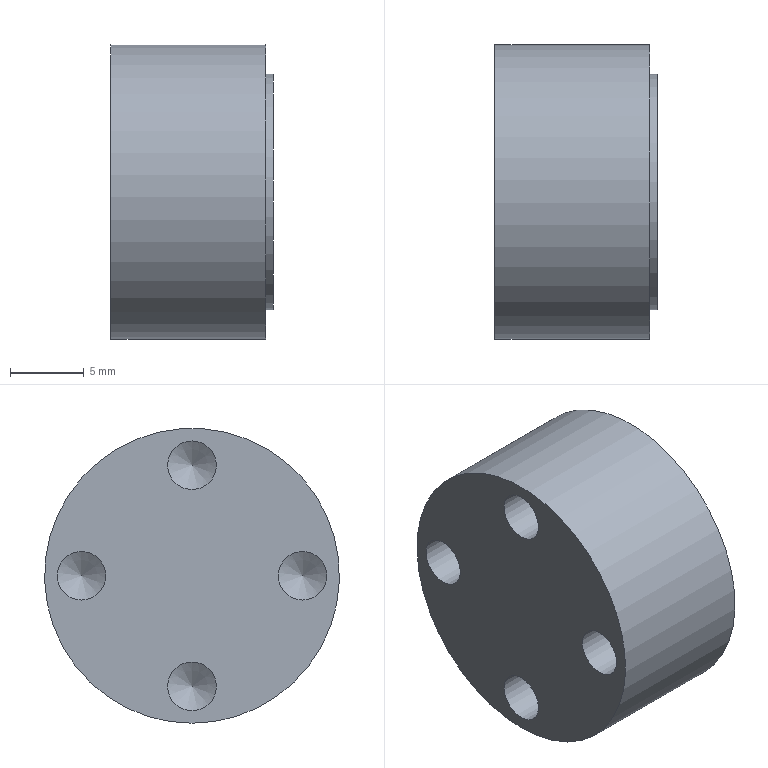Part | STEP file | Small compression-type pressure sensor LFC-20P | 1 solid | 13 faces | box 11 x 20 x 20 mm | volume 3302 mm3 | cylinder 6 | cone 4 | plane 3 | commonest cylinder face diameters 3.3 x4 16 x1 20 x1
STEP:
#1=CARTESIAN_POINT('',(10.5,0.,-10.));
#2=VERTEX_POINT('',#1);
#3=CARTESIAN_POINT('',(10.5,0.,0.));
#4=DIRECTION('',(1.,0.,0.));
#5=DIRECTION('',(0.,0.,-1.));
#6=AXIS2_PLACEMENT_3D('',#3,#4,#5);
#7=CIRCLE('',#6,10.);
#8=EDGE_CURVE('',#2,#2,#7,.T.);
#9=ORIENTED_EDGE('',*,*,#8,.F.);
#10=EDGE_LOOP('',(#9));
#11=FACE_OUTER_BOUND('',#10,.T.);
#12=CARTESIAN_POINT('',(0.,0.,-10.));
#13=VERTEX_POINT('',#12);
#14=CARTESIAN_POINT('',(0.,0.,0.));
#15=DIRECTION('',(1.,0.,0.));
#16=DIRECTION('',(0.,0.,-1.));
#17=AXIS2_PLACEMENT_3D('',#14,#15,#16);
#18=CIRCLE('',#17,10.);
#19=EDGE_CURVE('',#13,#13,#18,.T.);
#20=ORIENTED_EDGE('',*,*,#19,.T.);
#21=EDGE_LOOP('',(#20));
#22=FACE_OUTER_BOUND('',#21,.T.);
#23=CARTESIAN_POINT('',(10.5,0.,0.));
#24=DIRECTION('',(-1.,0.,0.));
#25=DIRECTION('',(0.,0.,1.));
#26=AXIS2_PLACEMENT_3D('',#23,#24,#25);
#27=CYLINDRICAL_SURFACE('',#26,10.);
#28=ADVANCED_FACE('',(#11,#22),#27,.T.);
#29=CARTESIAN_POINT('',(10.5,0.,-8.));
#30=VERTEX_POINT('',#29);
#31=CARTESIAN_POINT('',(10.5,0.,0.));
#32=DIRECTION('',(1.,0.,0.));
#33=DIRECTION('',(0.,0.,-1.));
#34=AXIS2_PLACEMENT_3D('',#31,#32,#33);
#35=CIRCLE('',#34,8.);
#36=EDGE_CURVE('',#30,#30,#35,.T.);
#37=ORIENTED_EDGE('',*,*,#36,.F.);
#38=EDGE_LOOP('',(#37));
#39=FACE_BOUND('',#38,.T.);
#40=ORIENTED_EDGE('',*,*,#8,.T.);
#41=EDGE_LOOP('',(#40));
#42=FACE_OUTER_BOUND('',#41,.T.);
#43=CARTESIAN_POINT('',(10.5,0.,0.));
#44=DIRECTION('',(1.,0.,0.));
#45=DIRECTION('',(0.,0.,-1.));
#46=AXIS2_PLACEMENT_3D('',#43,#44,#45);
#47=PLANE('',#46);
#48=ADVANCED_FACE('',(#39,#42),#47,.T.);
#49=CARTESIAN_POINT('',(0.,0.,-5.85));
#50=VERTEX_POINT('',#49);
#51=CARTESIAN_POINT('',(0.,0.,-7.5));
#52=DIRECTION('',(-1.,0.,0.));
#53=DIRECTION('',(0.,0.,1.));
#54=AXIS2_PLACEMENT_3D('',#51,#52,#53);
#55=CIRCLE('',#54,1.65);
#56=EDGE_CURVE('',#50,#50,#55,.T.);
#57=ORIENTED_EDGE('',*,*,#56,.F.);
#58=EDGE_LOOP('',(#57));
#59=FACE_BOUND('',#58,.T.);
#60=CARTESIAN_POINT('',(0.,7.5,1.65));
#61=VERTEX_POINT('',#60);
#62=CARTESIAN_POINT('',(0.,7.5,0.));
#63=DIRECTION('',(-1.,0.,0.));
#64=DIRECTION('',(0.,0.,1.));
#65=AXIS2_PLACEMENT_3D('',#62,#63,#64);
#66=CIRCLE('',#65,1.65);
#67=EDGE_CURVE('',#61,#61,#66,.T.);
#68=ORIENTED_EDGE('',*,*,#67,.F.);
#69=EDGE_LOOP('',(#68));
#70=FACE_BOUND('',#69,.T.);
#71=CARTESIAN_POINT('',(0.,0.,9.15));
#72=VERTEX_POINT('',#71);
#73=CARTESIAN_POINT('',(0.,0.,7.5));
#74=DIRECTION('',(-1.,0.,0.));
#75=DIRECTION('',(0.,0.,1.));
#76=AXIS2_PLACEMENT_3D('',#73,#74,#75);
#77=CIRCLE('',#76,1.65);
#78=EDGE_CURVE('',#72,#72,#77,.T.);
#79=ORIENTED_EDGE('',*,*,#78,.F.);
#80=EDGE_LOOP('',(#79));
#81=FACE_BOUND('',#80,.T.);
#82=CARTESIAN_POINT('',(0.,-7.5,1.65));
#83=VERTEX_POINT('',#82);
#84=CARTESIAN_POINT('',(0.,-7.5,0.));
#85=DIRECTION('',(-1.,0.,0.));
#86=DIRECTION('',(0.,0.,1.));
#87=AXIS2_PLACEMENT_3D('',#84,#85,#86);
#88=CIRCLE('',#87,1.65);
#89=EDGE_CURVE('',#83,#83,#88,.T.);
#90=ORIENTED_EDGE('',*,*,#89,.F.);
#91=EDGE_LOOP('',(#90));
#92=FACE_BOUND('',#91,.T.);
#93=ORIENTED_EDGE('',*,*,#19,.F.);
#94=EDGE_LOOP('',(#93));
#95=FACE_OUTER_BOUND('',#94,.T.);
#96=CARTESIAN_POINT('',(0.,0.,0.));
#97=DIRECTION('',(1.,0.,0.));
#98=DIRECTION('',(0.,0.,-1.));
#99=AXIS2_PLACEMENT_3D('',#96,#97,#98);
#100=PLANE('',#99);
#101=ADVANCED_FACE('',(#59,#70,#81,#92,#95),#100,.F.);
#102=CARTESIAN_POINT('',(11.,0.,-8.));
#103=VERTEX_POINT('',#102);
#104=CARTESIAN_POINT('',(11.,0.,0.));
#105=DIRECTION('',(1.,0.,0.));
#106=DIRECTION('',(0.,0.,-1.));
#107=AXIS2_PLACEMENT_3D('',#104,#105,#106);
#108=CIRCLE('',#107,8.);
#109=EDGE_CURVE('',#103,#103,#108,.T.);
#110=ORIENTED_EDGE('',*,*,#109,.F.);
#111=EDGE_LOOP('',(#110));
#112=FACE_OUTER_BOUND('',#111,.T.);
#113=ORIENTED_EDGE('',*,*,#36,.T.);
#114=EDGE_LOOP('',(#113));
#115=FACE_OUTER_BOUND('',#114,.T.);
#116=CARTESIAN_POINT('',(11.,0.,0.));
#117=DIRECTION('',(-1.,0.,0.));
#118=DIRECTION('',(0.,0.,1.));
#119=AXIS2_PLACEMENT_3D('',#116,#117,#118);
#120=CYLINDRICAL_SURFACE('',#119,8.);
#121=ADVANCED_FACE('',(#112,#115),#120,.T.);
#122=ORIENTED_EDGE('',*,*,#109,.T.);
#123=EDGE_LOOP('',(#122));
#124=FACE_OUTER_BOUND('',#123,.T.);
#125=CARTESIAN_POINT('',(11.,0.,0.));
#126=DIRECTION('',(1.,0.,0.));
#127=DIRECTION('',(0.,0.,-1.));
#128=AXIS2_PLACEMENT_3D('',#125,#126,#127);
#129=PLANE('',#128);
#130=ADVANCED_FACE('',(#124),#129,.T.);
#131=CARTESIAN_POINT('',(2.5,-7.5,1.65));
#132=VERTEX_POINT('',#131);
#133=CARTESIAN_POINT('',(2.5,-7.5,0.));
#134=DIRECTION('',(-1.,0.,0.));
#135=DIRECTION('',(0.,0.,1.));
#136=AXIS2_PLACEMENT_3D('',#133,#134,#135);
#137=CIRCLE('',#136,1.65);
#138=EDGE_CURVE('',#132,#132,#137,.T.);
#139=ORIENTED_EDGE('',*,*,#138,.T.);
#140=EDGE_LOOP('',(#139));
#141=FACE_OUTER_BOUND('',#140,.T.);
#142=CARTESIAN_POINT('',(2.5,-7.5,0.));
#143=DIRECTION('',(-1.,0.,0.));
#144=DIRECTION('',(0.,0.,1.));
#145=AXIS2_PLACEMENT_3D('',#142,#143,#144);
#146=CONICAL_SURFACE('',#145,1.65,1.03);
#147=ADVANCED_FACE('',(#141),#146,.F.);
#148=ORIENTED_EDGE('',*,*,#138,.F.);
#149=EDGE_LOOP('',(#148));
#150=FACE_OUTER_BOUND('',#149,.T.);
#151=ORIENTED_EDGE('',*,*,#89,.T.);
#152=EDGE_LOOP('',(#151));
#153=FACE_OUTER_BOUND('',#152,.T.);
#154=CARTESIAN_POINT('',(0.,-7.5,0.));
#155=DIRECTION('',(-1.,0.,0.));
#156=DIRECTION('',(0.,0.,1.));
#157=AXIS2_PLACEMENT_3D('',#154,#155,#156);
#158=CYLINDRICAL_SURFACE('',#157,1.65);
#159=ADVANCED_FACE('',(#150,#153),#158,.F.);
#160=CARTESIAN_POINT('',(2.5,0.,9.15));
#161=VERTEX_POINT('',#160);
#162=CARTESIAN_POINT('',(2.5,0.,7.5));
#163=DIRECTION('',(-1.,0.,0.));
#164=DIRECTION('',(0.,0.,1.));
#165=AXIS2_PLACEMENT_3D('',#162,#163,#164);
#166=CIRCLE('',#165,1.65);
#167=EDGE_CURVE('',#161,#161,#166,.T.);
#168=ORIENTED_EDGE('',*,*,#167,.T.);
#169=EDGE_LOOP('',(#168));
#170=FACE_OUTER_BOUND('',#169,.T.);
#171=CARTESIAN_POINT('',(2.5,0.,7.5));
#172=DIRECTION('',(-1.,0.,0.));
#173=DIRECTION('',(0.,0.,1.));
#174=AXIS2_PLACEMENT_3D('',#171,#172,#173);
#175=CONICAL_SURFACE('',#174,1.65,1.03);
#176=ADVANCED_FACE('',(#170),#175,.F.);
#177=ORIENTED_EDGE('',*,*,#167,.F.);
#178=EDGE_LOOP('',(#177));
#179=FACE_OUTER_BOUND('',#178,.T.);
#180=ORIENTED_EDGE('',*,*,#78,.T.);
#181=EDGE_LOOP('',(#180));
#182=FACE_OUTER_BOUND('',#181,.T.);
#183=CARTESIAN_POINT('',(0.,0.,7.5));
#184=DIRECTION('',(-1.,0.,0.));
#185=DIRECTION('',(0.,0.,1.));
#186=AXIS2_PLACEMENT_3D('',#183,#184,#185);
#187=CYLINDRICAL_SURFACE('',#186,1.65);
#188=ADVANCED_FACE('',(#179,#182),#187,.F.);
#189=CARTESIAN_POINT('',(2.5,7.5,1.65));
#190=VERTEX_POINT('',#189);
#191=CARTESIAN_POINT('',(2.5,7.5,0.));
#192=DIRECTION('',(-1.,0.,0.));
#193=DIRECTION('',(0.,0.,1.));
#194=AXIS2_PLACEMENT_3D('',#191,#192,#193);
#195=CIRCLE('',#194,1.65);
#196=EDGE_CURVE('',#190,#190,#195,.T.);
#197=ORIENTED_EDGE('',*,*,#196,.T.);
#198=EDGE_LOOP('',(#197));
#199=FACE_OUTER_BOUND('',#198,.T.);
#200=CARTESIAN_POINT('',(2.5,7.5,0.));
#201=DIRECTION('',(-1.,0.,0.));
#202=DIRECTION('',(0.,0.,1.));
#203=AXIS2_PLACEMENT_3D('',#200,#201,#202);
#204=CONICAL_SURFACE('',#203,1.65,1.03);
#205=ADVANCED_FACE('',(#199),#204,.F.);
#206=ORIENTED_EDGE('',*,*,#196,.F.);
#207=EDGE_LOOP('',(#206));
#208=FACE_OUTER_BOUND('',#207,.T.);
#209=ORIENTED_EDGE('',*,*,#67,.T.);
#210=EDGE_LOOP('',(#209));
#211=FACE_OUTER_BOUND('',#210,.T.);
#212=CARTESIAN_POINT('',(0.,7.5,0.));
#213=DIRECTION('',(-1.,0.,0.));
#214=DIRECTION('',(0.,0.,1.));
#215=AXIS2_PLACEMENT_3D('',#212,#213,#214);
#216=CYLINDRICAL_SURFACE('',#215,1.65);
#217=ADVANCED_FACE('',(#208,#211),#216,.F.);
#218=CARTESIAN_POINT('',(2.5,0.,-5.85));
#219=VERTEX_POINT('',#218);
#220=CARTESIAN_POINT('',(2.5,0.,-7.5));
#221=DIRECTION('',(-1.,0.,0.));
#222=DIRECTION('',(0.,0.,1.));
#223=AXIS2_PLACEMENT_3D('',#220,#221,#222);
#224=CIRCLE('',#223,1.65);
#225=EDGE_CURVE('',#219,#219,#224,.T.);
#226=ORIENTED_EDGE('',*,*,#225,.T.);
#227=EDGE_LOOP('',(#226));
#228=FACE_OUTER_BOUND('',#227,.T.);
#229=CARTESIAN_POINT('',(2.5,0.,-7.5));
#230=DIRECTION('',(-1.,0.,0.));
#231=DIRECTION('',(0.,0.,1.));
#232=AXIS2_PLACEMENT_3D('',#229,#230,#231);
#233=CONICAL_SURFACE('',#232,1.65,1.03);
#234=ADVANCED_FACE('',(#228),#233,.F.);
#235=ORIENTED_EDGE('',*,*,#225,.F.);
#236=EDGE_LOOP('',(#235));
#237=FACE_OUTER_BOUND('',#236,.T.);
#238=ORIENTED_EDGE('',*,*,#56,.T.);
#239=EDGE_LOOP('',(#238));
#240=FACE_OUTER_BOUND('',#239,.T.);
#241=CARTESIAN_POINT('',(0.,0.,-7.5));
#242=DIRECTION('',(-1.,0.,0.));
#243=DIRECTION('',(0.,0.,1.));
#244=AXIS2_PLACEMENT_3D('',#241,#242,#243);
#245=CYLINDRICAL_SURFACE('',#244,1.65);
#246=ADVANCED_FACE('',(#237,#240),#245,.F.);
#247=CLOSED_SHELL('',(#28,#48,#101,#121,#130,#147,#159,#176,#188,#205,#217,#234,#246));
#248=MANIFOLD_SOLID_BREP('',#247);
#249=CARTESIAN_POINT('',(0.,0.,0.));
#250=DIRECTION('',(0.,0.,1.));
#251=DIRECTION('',(1.,0.,0.));
#252=AXIS2_PLACEMENT_3D('',#249,#250,#251);
#253=(LENGTH_UNIT()NAMED_UNIT(*)SI_UNIT(.MILLI.,.METRE.));
#254=UNCERTAINTY_MEASURE_WITH_UNIT(LENGTH_MEASURE(0.00001),#253,'','');
#255=(NAMED_UNIT(*)PLANE_ANGLE_UNIT()SI_UNIT($,.RADIAN.));
#256=(NAMED_UNIT(*)SI_UNIT($,.STERADIAN.)SOLID_ANGLE_UNIT());
#257=(GEOMETRIC_REPRESENTATION_CONTEXT(3)GLOBAL_UNCERTAINTY_ASSIGNED_CONTEXT((#254))GLOBAL_UNIT_ASSIGNED_CONTEXT((#253,#255,#256))REPRESENTATION_CONTEXT('',''));
#258=ADVANCED_BREP_SHAPE_REPRESENTATION('',(#248,#252),#257);